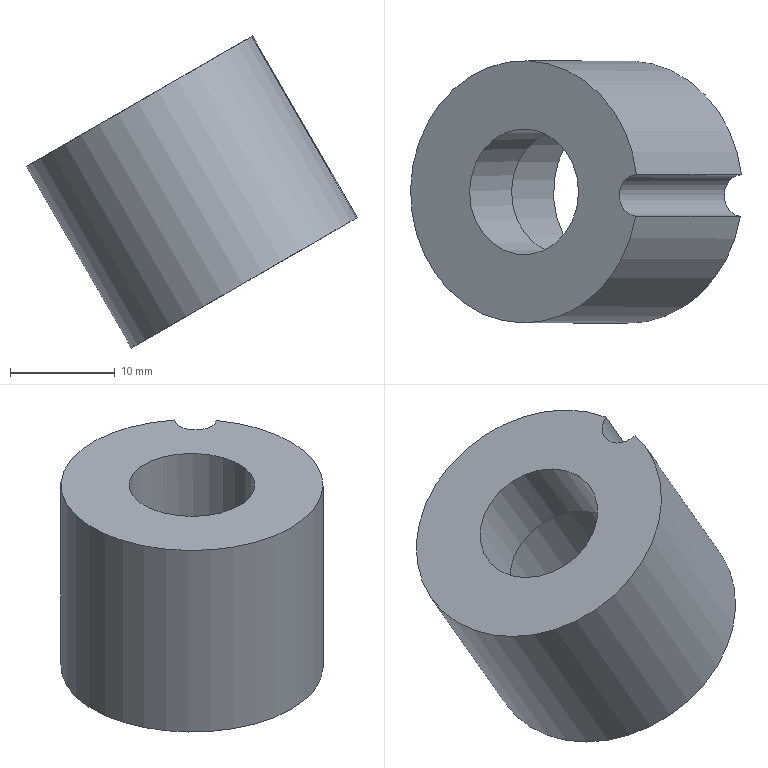Part | NX | features solid 2 | 1 solid | 7 faces | box 31.555 x 25 x 29.766 mm | volume 6194 mm3 | cylinder 4 | plane 3 | commonest cylinder face diameters 4 x1 12 x1 16.6 x1 25 x1
STEP:
#1=CARTESIAN_POINT('',(-239.371,135.654,29.174));
#2=VERTEX_POINT('',#1);
#3=CARTESIAN_POINT('',(-249.371,135.654,46.494));
#4=VERTEX_POINT('',#3);
#5=CARTESIAN_POINT('',(-244.371,135.654,37.834));
#6=DIRECTION('',(-0.5,0.,0.866));
#7=VECTOR('',#6,1000.);
#8=LINE('',#5,#7);
#9=EDGE_CURVE('',#2,#4,#8,.T.);
#10=ORIENTED_EDGE('',*,*,#9,.F.);
#11=CARTESIAN_POINT('',(-239.466,131.669,29.119));
#12=VERTEX_POINT('',#11);
#13=CARTESIAN_POINT('',(-250.101,134.,22.979));
#14=DIRECTION('',(-0.5,0.,0.866));
#15=DIRECTION('',(0.8657,-0.02744,0.4998));
#16=AXIS2_PLACEMENT_3D('',#13,#14,#15);
#17=CIRCLE('',#16,12.5);
#18=EDGE_CURVE('',#2,#12,#17,.T.);
#19=ORIENTED_EDGE('',*,*,#18,.T.);
#20=CARTESIAN_POINT('',(-249.466,131.669,46.44));
#21=VERTEX_POINT('',#20);
#22=CARTESIAN_POINT('',(-244.466,131.669,37.78));
#23=DIRECTION('',(-0.5,0.,0.866));
#24=VECTOR('',#23,1000.);
#25=LINE('',#22,#24);
#26=EDGE_CURVE('',#21,#12,#25,.F.);
#27=ORIENTED_EDGE('',*,*,#26,.F.);
#28=CARTESIAN_POINT('',(-260.101,134.,40.299));
#29=DIRECTION('',(-0.5,0.,0.866));
#30=DIRECTION('',(0.866,0.,0.5));
#31=AXIS2_PLACEMENT_3D('',#28,#29,#30);
#32=CIRCLE('',#31,12.5);
#33=EDGE_CURVE('',#4,#21,#32,.T.);
#34=ORIENTED_EDGE('',*,*,#33,.F.);
#35=EDGE_LOOP('',(#10,#19,#27,#34));
#36=FACE_BOUND('',#35,.T.);
#37=CARTESIAN_POINT('',(-250.101,134.,22.979));
#38=DIRECTION('',(-0.5,0.,0.866));
#39=DIRECTION('',(0.8657,-0.02744,0.4998));
#40=AXIS2_PLACEMENT_3D('',#37,#38,#39);
#41=CYLINDRICAL_SURFACE('',#40,12.5);
#42=ADVANCED_FACE('',(#36),#41,.T.);
#43=CARTESIAN_POINT('',(-242.916,133.772,27.127));
#44=VERTEX_POINT('',#43);
#45=CARTESIAN_POINT('',(-250.101,134.,22.979));
#46=DIRECTION('',(-0.5,0.,0.866));
#47=DIRECTION('',(0.8657,-0.02744,0.4998));
#48=AXIS2_PLACEMENT_3D('',#45,#46,#47);
#49=CIRCLE('',#48,8.3);
#50=EDGE_CURVE('',#44,#44,#49,.T.);
#51=ORIENTED_EDGE('',*,*,#50,.T.);
#52=EDGE_LOOP('',(#51));
#53=FACE_BOUND('',#52,.T.);
#54=ORIENTED_EDGE('',*,*,#18,.F.);
#55=CARTESIAN_POINT('',(-239.28,133.657,29.227));
#56=DIRECTION('',(-0.5,0.,0.866));
#57=DIRECTION('',(0.8657,-0.02744,0.4998));
#58=AXIS2_PLACEMENT_3D('',#55,#56,#57);
#59=CIRCLE('',#58,2.);
#60=EDGE_CURVE('',#2,#12,#59,.T.);
#61=ORIENTED_EDGE('',*,*,#60,.T.);
#62=EDGE_LOOP('',(#54,#61));
#63=FACE_BOUND('',#62,.T.);
#64=CARTESIAN_POINT('',(-250.101,134.,22.979));
#65=DIRECTION('',(-0.5,0.,0.866));
#66=DIRECTION('',(0.8657,-0.02744,0.4998));
#67=AXIS2_PLACEMENT_3D('',#64,#65,#66);
#68=PLANE('',#67);
#69=ADVANCED_FACE('',(#53,#63),#68,.F.);
#70=CARTESIAN_POINT('',(-254.905,134.,43.299));
#71=VERTEX_POINT('',#70);
#72=CARTESIAN_POINT('',(-260.101,134.,40.299));
#73=DIRECTION('',(-0.5,0.,0.866));
#74=DIRECTION('',(0.866,0.,0.5));
#75=AXIS2_PLACEMENT_3D('',#72,#73,#74);
#76=CIRCLE('',#75,6.);
#77=EDGE_CURVE('',#71,#71,#76,.T.);
#78=ORIENTED_EDGE('',*,*,#77,.F.);
#79=EDGE_LOOP('',(#78));
#80=FACE_BOUND('',#79,.T.);
#81=CARTESIAN_POINT('',(-249.28,133.657,46.547));
#82=DIRECTION('',(-0.5,0.,0.866));
#83=DIRECTION('',(0.866,0.,0.5));
#84=AXIS2_PLACEMENT_3D('',#81,#82,#83);
#85=CIRCLE('',#84,2.);
#86=EDGE_CURVE('',#4,#21,#85,.T.);
#87=ORIENTED_EDGE('',*,*,#86,.F.);
#88=ORIENTED_EDGE('',*,*,#33,.T.);
#89=EDGE_LOOP('',(#87,#88));
#90=FACE_BOUND('',#89,.T.);
#91=CARTESIAN_POINT('',(-260.101,134.,40.299));
#92=DIRECTION('',(-0.5,0.,0.866));
#93=DIRECTION('',(0.8657,-0.02744,0.4998));
#94=AXIS2_PLACEMENT_3D('',#91,#92,#93);
#95=PLANE('',#94);
#96=ADVANCED_FACE('',(#80,#90),#95,.T.);
#97=ORIENTED_EDGE('',*,*,#50,.F.);
#98=EDGE_LOOP('',(#97));
#99=FACE_BOUND('',#98,.T.);
#100=CARTESIAN_POINT('',(-248.916,133.772,37.52));
#101=VERTEX_POINT('',#100);
#102=CARTESIAN_POINT('',(-256.101,134.,33.371));
#103=DIRECTION('',(-0.5,0.,0.866));
#104=DIRECTION('',(0.8657,-0.02744,0.4998));
#105=AXIS2_PLACEMENT_3D('',#102,#103,#104);
#106=CIRCLE('',#105,8.3);
#107=EDGE_CURVE('',#101,#101,#106,.T.);
#108=ORIENTED_EDGE('',*,*,#107,.T.);
#109=EDGE_LOOP('',(#108));
#110=FACE_BOUND('',#109,.T.);
#111=CARTESIAN_POINT('',(-250.101,134.,22.979));
#112=DIRECTION('',(-0.5,0.,0.866));
#113=DIRECTION('',(0.8657,-0.02744,0.4998));
#114=AXIS2_PLACEMENT_3D('',#111,#112,#113);
#115=CYLINDRICAL_SURFACE('',#114,8.3);
#116=ADVANCED_FACE('',(#99,#110),#115,.F.);
#117=CARTESIAN_POINT('',(-250.907,133.835,36.37));
#118=VERTEX_POINT('',#117);
#119=CARTESIAN_POINT('',(-256.101,134.,33.371));
#120=DIRECTION('',(-0.5,0.,0.866));
#121=DIRECTION('',(0.8657,-0.02744,0.4998));
#122=AXIS2_PLACEMENT_3D('',#119,#120,#121);
#123=CIRCLE('',#122,6.);
#124=EDGE_CURVE('',#118,#118,#123,.T.);
#125=ORIENTED_EDGE('',*,*,#124,.T.);
#126=EDGE_LOOP('',(#125));
#127=FACE_BOUND('',#126,.T.);
#128=ORIENTED_EDGE('',*,*,#107,.F.);
#129=EDGE_LOOP('',(#128));
#130=FACE_BOUND('',#129,.T.);
#131=CARTESIAN_POINT('',(-256.101,134.,33.371));
#132=DIRECTION('',(-0.5,0.,0.866));
#133=DIRECTION('',(0.8657,-0.02744,0.4998));
#134=AXIS2_PLACEMENT_3D('',#131,#132,#133);
#135=PLANE('',#134);
#136=ADVANCED_FACE('',(#127,#130),#135,.F.);
#137=ORIENTED_EDGE('',*,*,#9,.T.);
#138=ORIENTED_EDGE('',*,*,#86,.T.);
#139=ORIENTED_EDGE('',*,*,#26,.T.);
#140=ORIENTED_EDGE('',*,*,#60,.F.);
#141=EDGE_LOOP('',(#137,#138,#139,#140));
#142=FACE_BOUND('',#141,.T.);
#143=CARTESIAN_POINT('',(-239.28,133.657,29.227));
#144=DIRECTION('',(-0.5,0.,0.866));
#145=DIRECTION('',(0.8657,-0.02744,0.4998));
#146=AXIS2_PLACEMENT_3D('',#143,#144,#145);
#147=CYLINDRICAL_SURFACE('',#146,2.);
#148=ADVANCED_FACE('',(#142),#147,.F.);
#149=ORIENTED_EDGE('',*,*,#77,.T.);
#150=EDGE_LOOP('',(#149));
#151=FACE_BOUND('',#150,.T.);
#152=ORIENTED_EDGE('',*,*,#124,.F.);
#153=EDGE_LOOP('',(#152));
#154=FACE_BOUND('',#153,.T.);
#155=CARTESIAN_POINT('',(-250.101,134.,22.979));
#156=DIRECTION('',(-0.5,0.,0.866));
#157=DIRECTION('',(0.8657,-0.02744,0.4998));
#158=AXIS2_PLACEMENT_3D('',#155,#156,#157);
#159=CYLINDRICAL_SURFACE('',#158,6.);
#160=ADVANCED_FACE('',(#151,#154),#159,.F.);
#161=CLOSED_SHELL('',(#42,#69,#96,#116,#136,#148,#160));
#162=MANIFOLD_SOLID_BREP('',#161);
#163=(LENGTH_UNIT()NAMED_UNIT(*)SI_UNIT(.MILLI.,.METRE.));
#164=UNCERTAINTY_MEASURE_WITH_UNIT(LENGTH_MEASURE(0.00001),#163,'','');
#165=(NAMED_UNIT(*)PLANE_ANGLE_UNIT()SI_UNIT($,.RADIAN.));
#166=(NAMED_UNIT(*)SI_UNIT($,.STERADIAN.)SOLID_ANGLE_UNIT());
#167=(GEOMETRIC_REPRESENTATION_CONTEXT(3)GLOBAL_UNCERTAINTY_ASSIGNED_CONTEXT((#164))GLOBAL_UNIT_ASSIGNED_CONTEXT((#163,#165,#166))REPRESENTATION_CONTEXT('',''));
#168=ADVANCED_BREP_SHAPE_REPRESENTATION('',(#162),#167);